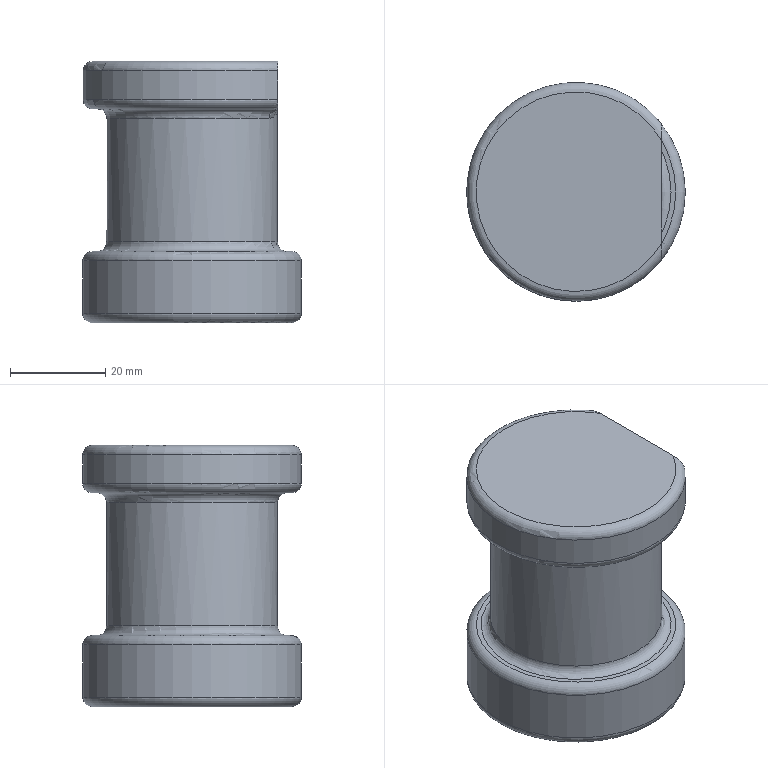Part | NX | features solid 2 | 1 solid | 19 faces | box 46 x 46 x 55 mm | volume 63111 mm3 | torus 6 | plane 5 | cylinder 4 | cone 2 | spline 2 | commonest cylinder face diameters 46 x2 14 x1 36 x1
STEP:
#1=CARTESIAN_POINT('',(458.,215.682,102.));
#2=VERTEX_POINT('',#1);
#3=CARTESIAN_POINT('',(458.,215.682,108.));
#4=VERTEX_POINT('',#3);
#5=CARTESIAN_POINT('',(458.,215.682,110.));
#6=DIRECTION('',(0.,0.,-1.));
#7=VECTOR('',#6,1000.);
#8=LINE('',#5,#7);
#9=EDGE_CURVE('',#2,#4,#8,.F.);
#10=ORIENTED_EDGE('',*,*,#9,.T.);
#11=CARTESIAN_POINT('',(458.,244.318,108.));
#12=VERTEX_POINT('',#11);
#13=CARTESIAN_POINT('',(440.,230.,108.));
#14=DIRECTION('',(0.,0.,1.));
#15=DIRECTION('',(1.,0.,0.));
#16=AXIS2_PLACEMENT_3D('',#13,#14,#15);
#17=CIRCLE('',#16,23.);
#18=EDGE_CURVE('',#12,#4,#17,.T.);
#19=ORIENTED_EDGE('',*,*,#18,.F.);
#20=CARTESIAN_POINT('',(458.,244.318,102.));
#21=VERTEX_POINT('',#20);
#22=CARTESIAN_POINT('',(458.,244.318,110.));
#23=DIRECTION('',(0.,0.,-1.));
#24=VECTOR('',#23,1000.);
#25=LINE('',#22,#24);
#26=EDGE_CURVE('',#12,#21,#25,.T.);
#27=ORIENTED_EDGE('',*,*,#26,.T.);
#28=CARTESIAN_POINT('',(440.,230.,102.));
#29=DIRECTION('',(0.,0.,1.));
#30=DIRECTION('',(1.,0.,0.));
#31=AXIS2_PLACEMENT_3D('',#28,#29,#30);
#32=CIRCLE('',#31,23.);
#33=EDGE_CURVE('',#2,#21,#32,.F.);
#34=ORIENTED_EDGE('',*,*,#33,.F.);
#35=EDGE_LOOP('',(#10,#19,#27,#34));
#36=FACE_BOUND('',#35,.T.);
#37=CARTESIAN_POINT('',(440.,230.,55.));
#38=DIRECTION('',(0.,0.,1.));
#39=DIRECTION('',(-1.,0.,0.));
#40=AXIS2_PLACEMENT_3D('',#37,#38,#39);
#41=CYLINDRICAL_SURFACE('',#40,23.);
#42=ADVANCED_FACE('',(#36),#41,.T.);
#43=CARTESIAN_POINT('',(458.,219.183,110.));
#44=VERTEX_POINT('',#43);
#45=CARTESIAN_POINT('',(458.,240.817,110.));
#46=VERTEX_POINT('',#45);
#47=CARTESIAN_POINT('',(458.,215.682,110.));
#48=DIRECTION('',(0.,1.,0.));
#49=VECTOR('',#48,1000.);
#50=LINE('',#47,#49);
#51=EDGE_CURVE('',#44,#46,#50,.T.);
#52=ORIENTED_EDGE('',*,*,#51,.T.);
#53=CARTESIAN_POINT('',(440.,230.,110.));
#54=DIRECTION('',(0.,0.,1.));
#55=DIRECTION('',(1.,0.,0.));
#56=AXIS2_PLACEMENT_3D('',#53,#54,#55);
#57=CIRCLE('',#56,21.);
#58=EDGE_CURVE('',#44,#46,#57,.F.);
#59=ORIENTED_EDGE('',*,*,#58,.F.);
#60=EDGE_LOOP('',(#52,#59));
#61=FACE_BOUND('',#60,.T.);
#62=CARTESIAN_POINT('',(440.,230.,110.));
#63=DIRECTION('',(0.,0.,-1.));
#64=DIRECTION('',(1.,0.,0.));
#65=AXIS2_PLACEMENT_3D('',#62,#63,#64);
#66=PLANE('',#65);
#67=ADVANCED_FACE('',(#61),#66,.F.);
#68=CARTESIAN_POINT('',(458.,219.183,100.));
#69=VERTEX_POINT('',#68);
#70=CARTESIAN_POINT('',(458.,221.282,100.));
#71=VERTEX_POINT('',#70);
#72=CARTESIAN_POINT('',(458.,230.,100.));
#73=DIRECTION('',(0.,1.,0.));
#74=VECTOR('',#73,1000.);
#75=LINE('',#72,#74);
#76=EDGE_CURVE('',#69,#71,#75,.T.);
#77=ORIENTED_EDGE('',*,*,#76,.F.);
#78=CARTESIAN_POINT('',(458.,240.817,100.));
#79=VERTEX_POINT('',#78);
#80=CARTESIAN_POINT('',(440.,230.,100.));
#81=DIRECTION('',(0.,0.,1.));
#82=DIRECTION('',(1.,0.,0.));
#83=AXIS2_PLACEMENT_3D('',#80,#81,#82);
#84=CIRCLE('',#83,21.);
#85=EDGE_CURVE('',#79,#69,#84,.T.);
#86=ORIENTED_EDGE('',*,*,#85,.F.);
#87=CARTESIAN_POINT('',(458.,238.718,100.));
#88=VERTEX_POINT('',#87);
#89=CARTESIAN_POINT('',(458.,230.,100.));
#90=DIRECTION('',(0.,1.,0.));
#91=VECTOR('',#90,1000.);
#92=LINE('',#89,#91);
#93=EDGE_CURVE('',#88,#79,#92,.T.);
#94=ORIENTED_EDGE('',*,*,#93,.F.);
#95=CARTESIAN_POINT('',(440.,230.,100.));
#96=DIRECTION('',(0.,0.,1.));
#97=DIRECTION('',(1.,0.,0.));
#98=AXIS2_PLACEMENT_3D('',#95,#96,#97);
#99=CIRCLE('',#98,20.);
#100=EDGE_CURVE('',#71,#88,#99,.F.);
#101=ORIENTED_EDGE('',*,*,#100,.F.);
#102=EDGE_LOOP('',(#77,#86,#94,#101));
#103=FACE_BOUND('',#102,.T.);
#104=CARTESIAN_POINT('',(440.,230.,100.));
#105=DIRECTION('',(0.,0.,-1.));
#106=DIRECTION('',(0.,-1.,0.));
#107=AXIS2_PLACEMENT_3D('',#104,#105,#106);
#108=PLANE('',#107);
#109=ADVANCED_FACE('',(#103),#108,.T.);
#110=ORIENTED_EDGE('',*,*,#58,.T.);
#111=CARTESIAN_POINT('',(458.,244.318,108.));
#112=CARTESIAN_POINT('',(458.,244.318,108.369));
#113=CARTESIAN_POINT('',(458.,243.958,109.078));
#114=CARTESIAN_POINT('',(458.,242.663,109.852));
#115=CARTESIAN_POINT('',(458.,241.547,110.));
#116=CARTESIAN_POINT('',(458.,240.817,110.));
#117=B_SPLINE_CURVE_WITH_KNOTS('',3,(#111,#112,#113,#114,#115,#116),.UNSPECIFIED.,.F.,.F.,(4,1,1,4),(0.01075,0.01186,0.01296,0.01517),.UNSPECIFIED.);
#118=EDGE_CURVE('',#12,#46,#117,.T.);
#119=ORIENTED_EDGE('',*,*,#118,.F.);
#120=ORIENTED_EDGE('',*,*,#18,.T.);
#121=CARTESIAN_POINT('',(458.,219.183,110.));
#122=CARTESIAN_POINT('',(458.,218.445,110.));
#123=CARTESIAN_POINT('',(458.,217.331,109.849));
#124=CARTESIAN_POINT('',(458.,216.044,109.077));
#125=CARTESIAN_POINT('',(458.,215.682,108.374));
#126=CARTESIAN_POINT('',(458.,215.682,108.));
#127=B_SPLINE_CURVE_WITH_KNOTS('',3,(#121,#122,#123,#124,#125,#126),.UNSPECIFIED.,.F.,.F.,(4,1,1,4),(0.01631,0.01853,0.01964,0.02075),.UNSPECIFIED.);
#128=EDGE_CURVE('',#44,#4,#127,.T.);
#129=ORIENTED_EDGE('',*,*,#128,.F.);
#130=EDGE_LOOP('',(#110,#119,#120,#129));
#131=FACE_BOUND('',#130,.T.);
#132=CARTESIAN_POINT('',(440.,230.,108.));
#133=DIRECTION('',(0.,0.,-1.));
#134=DIRECTION('',(1.,0.,0.));
#135=AXIS2_PLACEMENT_3D('',#132,#133,#134);
#136=TOROIDAL_SURFACE('',#135,21.,2.);
#137=ADVANCED_FACE('',(#131),#136,.T.);
#138=CARTESIAN_POINT('',(460.,230.,70.));
#139=VERTEX_POINT('',#138);
#140=CARTESIAN_POINT('',(440.,230.,70.));
#141=DIRECTION('',(0.,0.,1.));
#142=DIRECTION('',(1.,0.,0.));
#143=AXIS2_PLACEMENT_3D('',#140,#141,#142);
#144=CIRCLE('',#143,20.);
#145=EDGE_CURVE('',#139,#139,#144,.T.);
#146=ORIENTED_EDGE('',*,*,#145,.F.);
#147=EDGE_LOOP('',(#146));
#148=FACE_BOUND('',#147,.T.);
#149=CARTESIAN_POINT('',(461.,230.,70.));
#150=VERTEX_POINT('',#149);
#151=CARTESIAN_POINT('',(440.,230.,70.));
#152=DIRECTION('',(0.,0.,1.));
#153=DIRECTION('',(1.,0.,0.));
#154=AXIS2_PLACEMENT_3D('',#151,#152,#153);
#155=CIRCLE('',#154,21.);
#156=EDGE_CURVE('',#150,#150,#155,.F.);
#157=ORIENTED_EDGE('',*,*,#156,.F.);
#158=EDGE_LOOP('',(#157));
#159=FACE_BOUND('',#158,.T.);
#160=CARTESIAN_POINT('',(440.,230.,70.));
#161=DIRECTION('',(0.,0.,-1.));
#162=DIRECTION('',(0.,-1.,0.));
#163=AXIS2_PLACEMENT_3D('',#160,#161,#162);
#164=PLANE('',#163);
#165=ADVANCED_FACE('',(#148,#159),#164,.F.);
#166=CARTESIAN_POINT('',(458.,230.,72.));
#167=VERTEX_POINT('',#166);
#168=CARTESIAN_POINT('',(440.,230.,72.));
#169=DIRECTION('',(0.,0.,1.));
#170=DIRECTION('',(1.,0.,0.));
#171=AXIS2_PLACEMENT_3D('',#168,#169,#170);
#172=CIRCLE('',#171,18.);
#173=EDGE_CURVE('',#167,#167,#172,.F.);
#174=ORIENTED_EDGE('',*,*,#173,.F.);
#175=EDGE_LOOP('',(#174));
#176=FACE_BOUND('',#175,.T.);
#177=CARTESIAN_POINT('',(456.2,222.154,98.));
#178=VERTEX_POINT('',#177);
#179=CARTESIAN_POINT('',(458.,230.,100.));
#180=VERTEX_POINT('',#179);
#181=CARTESIAN_POINT('',(456.2,222.154,98.));
#182=CARTESIAN_POINT('',(456.817,223.428,98.));
#183=CARTESIAN_POINT('',(457.712,226.043,98.614));
#184=CARTESIAN_POINT('',(458.,228.665,99.531));
#185=CARTESIAN_POINT('',(458.,230.,100.));
#186=B_SPLINE_CURVE_WITH_KNOTS('',3,(#181,#182,#183,#184,#185),.UNSPECIFIED.,.F.,.F.,(4,1,4),(0.,0.004245,0.00849),.UNSPECIFIED.);
#187=EDGE_CURVE('',#178,#180,#186,.T.);
#188=ORIENTED_EDGE('',*,*,#187,.F.);
#189=CARTESIAN_POINT('',(456.2,237.846,98.));
#190=VERTEX_POINT('',#189);
#191=CARTESIAN_POINT('',(440.,230.,98.));
#192=DIRECTION('',(0.,0.,1.));
#193=DIRECTION('',(1.,0.,0.));
#194=AXIS2_PLACEMENT_3D('',#191,#192,#193);
#195=CIRCLE('',#194,18.);
#196=EDGE_CURVE('',#190,#178,#195,.T.);
#197=ORIENTED_EDGE('',*,*,#196,.F.);
#198=CARTESIAN_POINT('',(456.2,237.846,98.));
#199=CARTESIAN_POINT('',(456.817,236.572,98.));
#200=CARTESIAN_POINT('',(457.712,233.957,98.614));
#201=CARTESIAN_POINT('',(458.,231.335,99.531));
#202=CARTESIAN_POINT('',(458.,230.,100.));
#203=B_SPLINE_CURVE_WITH_KNOTS('',3,(#198,#199,#200,#201,#202),.UNSPECIFIED.,.F.,.F.,(4,1,4),(0.,0.004245,0.00849),.UNSPECIFIED.);
#204=EDGE_CURVE('',#180,#190,#203,.F.);
#205=ORIENTED_EDGE('',*,*,#204,.F.);
#206=EDGE_LOOP('',(#188,#197,#205));
#207=FACE_BOUND('',#206,.T.);
#208=CARTESIAN_POINT('',(440.,230.,85.));
#209=DIRECTION('',(0.,0.,-1.));
#210=DIRECTION('',(0.,-1.,0.));
#211=AXIS2_PLACEMENT_3D('',#208,#209,#210);
#212=CYLINDRICAL_SURFACE('',#211,18.);
#213=ADVANCED_FACE('',(#176,#207),#212,.T.);
#214=CARTESIAN_POINT('',(461.,230.,55.));
#215=VERTEX_POINT('',#214);
#216=CARTESIAN_POINT('',(440.,230.,55.));
#217=DIRECTION('',(0.,0.,1.));
#218=DIRECTION('',(1.,0.,0.));
#219=AXIS2_PLACEMENT_3D('',#216,#217,#218);
#220=CIRCLE('',#219,21.);
#221=EDGE_CURVE('',#215,#215,#220,.T.);
#222=ORIENTED_EDGE('',*,*,#221,.F.);
#223=EDGE_LOOP('',(#222));
#224=FACE_BOUND('',#223,.T.);
#225=CARTESIAN_POINT('',(429.,230.,55.));
#226=VERTEX_POINT('',#225);
#227=CARTESIAN_POINT('',(440.,230.,55.));
#228=DIRECTION('',(0.,0.,-1.));
#229=DIRECTION('',(-1.,0.,0.));
#230=AXIS2_PLACEMENT_3D('',#227,#228,#229);
#231=CIRCLE('',#230,11.);
#232=EDGE_CURVE('',#226,#226,#231,.T.);
#233=ORIENTED_EDGE('',*,*,#232,.F.);
#234=EDGE_LOOP('',(#233));
#235=FACE_BOUND('',#234,.T.);
#236=CARTESIAN_POINT('',(440.,230.,55.));
#237=DIRECTION('',(0.,0.,-1.));
#238=DIRECTION('',(1.,0.,0.));
#239=AXIS2_PLACEMENT_3D('',#236,#237,#238);
#240=PLANE('',#239);
#241=ADVANCED_FACE('',(#224,#235),#240,.T.);
#242=CARTESIAN_POINT('',(463.,230.,57.));
#243=VERTEX_POINT('',#242);
#244=CARTESIAN_POINT('',(440.,230.,57.));
#245=DIRECTION('',(0.,0.,1.));
#246=DIRECTION('',(1.,0.,0.));
#247=AXIS2_PLACEMENT_3D('',#244,#245,#246);
#248=CIRCLE('',#247,23.);
#249=EDGE_CURVE('',#243,#243,#248,.F.);
#250=ORIENTED_EDGE('',*,*,#249,.F.);
#251=EDGE_LOOP('',(#250));
#252=FACE_BOUND('',#251,.T.);
#253=CARTESIAN_POINT('',(463.,230.,68.));
#254=VERTEX_POINT('',#253);
#255=CARTESIAN_POINT('',(440.,230.,68.));
#256=DIRECTION('',(0.,0.,1.));
#257=DIRECTION('',(1.,0.,0.));
#258=AXIS2_PLACEMENT_3D('',#255,#256,#257);
#259=CIRCLE('',#258,23.);
#260=EDGE_CURVE('',#254,#254,#259,.T.);
#261=ORIENTED_EDGE('',*,*,#260,.F.);
#262=EDGE_LOOP('',(#261));
#263=FACE_BOUND('',#262,.T.);
#264=CARTESIAN_POINT('',(440.,230.,55.));
#265=DIRECTION('',(0.,0.,1.));
#266=DIRECTION('',(-1.,0.,0.));
#267=AXIS2_PLACEMENT_3D('',#264,#265,#266);
#268=CYLINDRICAL_SURFACE('',#267,23.);
#269=ADVANCED_FACE('',(#252,#263),#268,.T.);
#270=CARTESIAN_POINT('',(433.,230.,100.));
#271=VERTEX_POINT('',#270);
#272=CARTESIAN_POINT('',(440.,230.,100.));
#273=DIRECTION('',(0.,0.,-1.));
#274=DIRECTION('',(-1.,0.,0.));
#275=AXIS2_PLACEMENT_3D('',#272,#273,#274);
#276=CIRCLE('',#275,7.);
#277=EDGE_CURVE('',#271,#271,#276,.T.);
#278=ORIENTED_EDGE('',*,*,#277,.T.);
#279=EDGE_LOOP('',(#278));
#280=FACE_BOUND('',#279,.T.);
#281=CARTESIAN_POINT('',(440.,230.,101.876));
#282=VERTEX_POINT('',#281);
#283=VERTEX_LOOP('',#282);
#284=FACE_BOUND('',#283,.T.);
#285=CARTESIAN_POINT('',(440.,230.,100.));
#286=DIRECTION('',(0.,0.,-1.));
#287=DIRECTION('',(1.,0.,0.));
#288=AXIS2_PLACEMENT_3D('',#285,#286,#287);
#289=CONICAL_SURFACE('',#288,7.,1.309);
#290=ADVANCED_FACE('',(#280,#284),#289,.F.);
#291=ORIENTED_EDGE('',*,*,#277,.F.);
#292=EDGE_LOOP('',(#291));
#293=FACE_BOUND('',#292,.T.);
#294=CARTESIAN_POINT('',(433.,230.,61.928));
#295=VERTEX_POINT('',#294);
#296=CARTESIAN_POINT('',(440.,230.,61.928));
#297=DIRECTION('',(0.,0.,-1.));
#298=DIRECTION('',(-1.,0.,0.));
#299=AXIS2_PLACEMENT_3D('',#296,#297,#298);
#300=CIRCLE('',#299,7.);
#301=EDGE_CURVE('',#295,#295,#300,.T.);
#302=ORIENTED_EDGE('',*,*,#301,.T.);
#303=EDGE_LOOP('',(#302));
#304=FACE_BOUND('',#303,.T.);
#305=CARTESIAN_POINT('',(440.,230.,100.));
#306=DIRECTION('',(0.,0.,1.));
#307=DIRECTION('',(-1.,0.,0.));
#308=AXIS2_PLACEMENT_3D('',#305,#306,#307);
#309=CYLINDRICAL_SURFACE('',#308,7.);
#310=ADVANCED_FACE('',(#293,#304),#309,.F.);
#311=ORIENTED_EDGE('',*,*,#301,.F.);
#312=EDGE_LOOP('',(#311));
#313=FACE_BOUND('',#312,.T.);
#314=ORIENTED_EDGE('',*,*,#232,.T.);
#315=EDGE_LOOP('',(#314));
#316=FACE_BOUND('',#315,.T.);
#317=CARTESIAN_POINT('',(440.,230.,55.));
#318=DIRECTION('',(0.,0.,-1.));
#319=DIRECTION('',(1.,0.,0.));
#320=AXIS2_PLACEMENT_3D('',#317,#318,#319);
#321=CONICAL_SURFACE('',#320,11.,0.5236);
#322=ADVANCED_FACE('',(#313,#316),#321,.F.);
#323=ORIENTED_EDGE('',*,*,#76,.T.);
#324=CARTESIAN_POINT('',(458.,230.,100.));
#325=DIRECTION('',(0.,1.,0.));
#326=VECTOR('',#325,1000.);
#327=LINE('',#324,#326);
#328=EDGE_CURVE('',#71,#180,#327,.T.);
#329=ORIENTED_EDGE('',*,*,#328,.T.);
#330=CARTESIAN_POINT('',(458.,230.,100.));
#331=DIRECTION('',(0.,1.,0.));
#332=VECTOR('',#331,1000.);
#333=LINE('',#330,#332);
#334=EDGE_CURVE('',#180,#88,#333,.T.);
#335=ORIENTED_EDGE('',*,*,#334,.T.);
#336=ORIENTED_EDGE('',*,*,#93,.T.);
#337=CARTESIAN_POINT('',(458.,244.318,102.));
#338=CARTESIAN_POINT('',(458.,244.318,101.625));
#339=CARTESIAN_POINT('',(458.,243.959,100.927));
#340=CARTESIAN_POINT('',(458.,242.668,100.149));
#341=CARTESIAN_POINT('',(458.,241.556,100.));
#342=CARTESIAN_POINT('',(458.,240.817,100.));
#343=B_SPLINE_CURVE_WITH_KNOTS('',3,(#337,#338,#339,#340,#341,#342),.UNSPECIFIED.,.F.,.F.,(4,1,1,4),(0.,0.001103,0.002207,0.004413),.UNSPECIFIED.);
#344=EDGE_CURVE('',#21,#79,#343,.T.);
#345=ORIENTED_EDGE('',*,*,#344,.F.);
#346=ORIENTED_EDGE('',*,*,#26,.F.);
#347=ORIENTED_EDGE('',*,*,#118,.T.);
#348=ORIENTED_EDGE('',*,*,#51,.F.);
#349=ORIENTED_EDGE('',*,*,#128,.T.);
#350=ORIENTED_EDGE('',*,*,#9,.F.);
#351=CARTESIAN_POINT('',(458.,219.183,100.));
#352=CARTESIAN_POINT('',(458.,218.444,100.));
#353=CARTESIAN_POINT('',(458.,217.342,100.145));
#354=CARTESIAN_POINT('',(458.,216.042,100.925));
#355=CARTESIAN_POINT('',(458.,215.682,101.625));
#356=CARTESIAN_POINT('',(458.,215.682,102.));
#357=B_SPLINE_CURVE_WITH_KNOTS('',3,(#351,#352,#353,#354,#355,#356),.UNSPECIFIED.,.F.,.F.,(4,1,1,4),(0.,0.002188,0.003282,0.004376),.UNSPECIFIED.);
#358=EDGE_CURVE('',#69,#2,#357,.T.);
#359=ORIENTED_EDGE('',*,*,#358,.F.);
#360=EDGE_LOOP('',(#323,#329,#335,#336,#345,#346,#347,#348,#349,#350,#359));
#361=FACE_BOUND('',#360,.T.);
#362=CARTESIAN_POINT('',(458.,215.682,110.));
#363=DIRECTION('',(1.,0.,0.));
#364=DIRECTION('',(0.,0.,1.));
#365=AXIS2_PLACEMENT_3D('',#362,#363,#364);
#366=PLANE('',#365);
#367=ADVANCED_FACE('',(#361),#366,.T.);
#368=ORIENTED_EDGE('',*,*,#249,.T.);
#369=EDGE_LOOP('',(#368));
#370=FACE_BOUND('',#369,.T.);
#371=ORIENTED_EDGE('',*,*,#221,.T.);
#372=EDGE_LOOP('',(#371));
#373=FACE_BOUND('',#372,.T.);
#374=CARTESIAN_POINT('',(440.,230.,57.));
#375=DIRECTION('',(0.,0.,-1.));
#376=DIRECTION('',(1.,0.,0.));
#377=AXIS2_PLACEMENT_3D('',#374,#375,#376);
#378=TOROIDAL_SURFACE('',#377,21.,2.);
#379=ADVANCED_FACE('',(#370,#373),#378,.T.);
#380=ORIENTED_EDGE('',*,*,#328,.F.);
#381=CARTESIAN_POINT('',(458.,221.282,98.));
#382=DIRECTION('',(0.4359,0.9,0.));
#383=DIRECTION('',(-0.9,0.4359,0.));
#384=AXIS2_PLACEMENT_3D('',#381,#382,#383);
#385=CIRCLE('',#384,2.);
#386=EDGE_CURVE('',#71,#178,#385,.F.);
#387=ORIENTED_EDGE('',*,*,#386,.T.);
#388=ORIENTED_EDGE('',*,*,#187,.T.);
#389=EDGE_LOOP('',(#380,#387,#388));
#390=FACE_BOUND('',#389,.T.);
#391=CARTESIAN_POINT('',(458.,221.282,100.));
#392=CARTESIAN_POINT('',(456.2,222.154,100.));
#393=CARTESIAN_POINT('',(456.2,222.154,98.));
#394=CARTESIAN_POINT('',(458.,222.683,100.));
#395=CARTESIAN_POINT('',(456.618,223.017,99.47));
#396=CARTESIAN_POINT('',(456.81,223.414,98.));
#397=CARTESIAN_POINT('',(458.,225.584,100.));
#398=CARTESIAN_POINT('',(457.644,225.617,99.263));
#399=CARTESIAN_POINT('',(457.709,226.026,98.608));
#400=CARTESIAN_POINT('',(458.,228.515,100.));
#401=CARTESIAN_POINT('',(458.,228.59,99.765));
#402=CARTESIAN_POINT('',(458.,228.664,99.531));
#403=CARTESIAN_POINT('',(458.,230.,100.));
#404=CARTESIAN_POINT('',(458.,230.,100.));
#405=CARTESIAN_POINT('',(458.,230.,100.));
#406=(BOUNDED_SURFACE()B_SPLINE_SURFACE(3,2,((#391,#392,#393),(#394,#395,#396),(#397,#398,#399),(#400,#401,#402),(#403,#404,#405)),.UNSPECIFIED.,.F.,.F.,.F.)B_SPLINE_SURFACE_WITH_KNOTS((4,1,4),(3,3),(0.004746,0.009418,0.01409),(0.,1.),.UNSPECIFIED.)GEOMETRIC_REPRESENTATION_ITEM()RATIONAL_B_SPLINE_SURFACE(((1.,0.7071,1.),(1.,0.815,1.),(1.,0.9556,1.),(1.,1.,1.),(1.,1.,1.)))REPRESENTATION_ITEM('')SURFACE());
#407=ADVANCED_FACE('',(#390),#406,.F.);
#408=ORIENTED_EDGE('',*,*,#386,.F.);
#409=ORIENTED_EDGE('',*,*,#100,.T.);
#410=CARTESIAN_POINT('',(458.,238.718,98.));
#411=DIRECTION('',(0.4359,-0.9,0.));
#412=DIRECTION('',(0.9,0.4359,0.));
#413=AXIS2_PLACEMENT_3D('',#410,#411,#412);
#414=CIRCLE('',#413,2.);
#415=EDGE_CURVE('',#88,#190,#414,.T.);
#416=ORIENTED_EDGE('',*,*,#415,.T.);
#417=ORIENTED_EDGE('',*,*,#196,.T.);
#418=EDGE_LOOP('',(#408,#409,#416,#417));
#419=FACE_BOUND('',#418,.T.);
#420=CARTESIAN_POINT('',(440.,230.,98.));
#421=DIRECTION('',(0.,0.,-1.));
#422=DIRECTION('',(1.,0.,0.));
#423=AXIS2_PLACEMENT_3D('',#420,#421,#422);
#424=TOROIDAL_SURFACE('',#423,20.,2.);
#425=ADVANCED_FACE('',(#419),#424,.F.);
#426=ORIENTED_EDGE('',*,*,#204,.T.);
#427=ORIENTED_EDGE('',*,*,#415,.F.);
#428=ORIENTED_EDGE('',*,*,#334,.F.);
#429=EDGE_LOOP('',(#426,#427,#428));
#430=FACE_BOUND('',#429,.T.);
#431=CARTESIAN_POINT('',(456.2,237.846,98.));
#432=CARTESIAN_POINT('',(456.2,237.846,100.));
#433=CARTESIAN_POINT('',(458.,238.718,100.));
#434=CARTESIAN_POINT('',(456.81,236.586,98.));
#435=CARTESIAN_POINT('',(456.618,236.983,99.47));
#436=CARTESIAN_POINT('',(458.,237.317,100.));
#437=CARTESIAN_POINT('',(457.709,233.974,98.608));
#438=CARTESIAN_POINT('',(457.644,234.383,99.263));
#439=CARTESIAN_POINT('',(458.,234.416,100.));
#440=CARTESIAN_POINT('',(458.,231.336,99.531));
#441=CARTESIAN_POINT('',(458.,231.41,99.765));
#442=CARTESIAN_POINT('',(458.,231.485,100.));
#443=CARTESIAN_POINT('',(458.,230.,100.));
#444=CARTESIAN_POINT('',(458.,230.,100.));
#445=CARTESIAN_POINT('',(458.,230.,100.));
#446=(BOUNDED_SURFACE()B_SPLINE_SURFACE(3,2,((#431,#432,#433),(#434,#435,#436),(#437,#438,#439),(#440,#441,#442),(#443,#444,#445)),.UNSPECIFIED.,.F.,.F.,.F.)B_SPLINE_SURFACE_WITH_KNOTS((4,1,4),(3,3),(0.004746,0.009418,0.01409),(0.,1.),.UNSPECIFIED.)GEOMETRIC_REPRESENTATION_ITEM()RATIONAL_B_SPLINE_SURFACE(((1.,0.7071,1.),(1.,0.815,1.),(1.,0.9556,1.),(1.,1.,1.),(1.,1.,1.)))REPRESENTATION_ITEM('')SURFACE());
#447=ADVANCED_FACE('',(#430),#446,.F.);
#448=ORIENTED_EDGE('',*,*,#344,.T.);
#449=ORIENTED_EDGE('',*,*,#85,.T.);
#450=ORIENTED_EDGE('',*,*,#358,.T.);
#451=ORIENTED_EDGE('',*,*,#33,.T.);
#452=EDGE_LOOP('',(#448,#449,#450,#451));
#453=FACE_BOUND('',#452,.T.);
#454=CARTESIAN_POINT('',(440.,230.,102.));
#455=DIRECTION('',(0.,0.,-1.));
#456=DIRECTION('',(1.,0.,0.));
#457=AXIS2_PLACEMENT_3D('',#454,#455,#456);
#458=TOROIDAL_SURFACE('',#457,21.,2.);
#459=ADVANCED_FACE('',(#453),#458,.T.);
#460=ORIENTED_EDGE('',*,*,#173,.T.);
#461=EDGE_LOOP('',(#460));
#462=FACE_BOUND('',#461,.T.);
#463=ORIENTED_EDGE('',*,*,#145,.T.);
#464=EDGE_LOOP('',(#463));
#465=FACE_BOUND('',#464,.T.);
#466=CARTESIAN_POINT('',(440.,230.,72.));
#467=DIRECTION('',(0.,0.,-1.));
#468=DIRECTION('',(1.,0.,0.));
#469=AXIS2_PLACEMENT_3D('',#466,#467,#468);
#470=TOROIDAL_SURFACE('',#469,20.,2.);
#471=ADVANCED_FACE('',(#462,#465),#470,.F.);
#472=ORIENTED_EDGE('',*,*,#156,.T.);
#473=EDGE_LOOP('',(#472));
#474=FACE_BOUND('',#473,.T.);
#475=ORIENTED_EDGE('',*,*,#260,.T.);
#476=EDGE_LOOP('',(#475));
#477=FACE_BOUND('',#476,.T.);
#478=CARTESIAN_POINT('',(440.,230.,68.));
#479=DIRECTION('',(0.,0.,-1.));
#480=DIRECTION('',(1.,0.,0.));
#481=AXIS2_PLACEMENT_3D('',#478,#479,#480);
#482=TOROIDAL_SURFACE('',#481,21.,2.);
#483=ADVANCED_FACE('',(#474,#477),#482,.T.);
#484=CLOSED_SHELL('',(#42,#67,#109,#137,#165,#213,#241,#269,#290,#310,#322,#367,#379,#407,#425,#447,#459,#471,#483));
#485=MANIFOLD_SOLID_BREP('',#484);
#486=(LENGTH_UNIT()NAMED_UNIT(*)SI_UNIT(.MILLI.,.METRE.));
#487=UNCERTAINTY_MEASURE_WITH_UNIT(LENGTH_MEASURE(0.0508),#486,'','');
#488=(NAMED_UNIT(*)PLANE_ANGLE_UNIT()SI_UNIT($,.RADIAN.));
#489=(NAMED_UNIT(*)SI_UNIT($,.STERADIAN.)SOLID_ANGLE_UNIT());
#490=(GEOMETRIC_REPRESENTATION_CONTEXT(3)GLOBAL_UNCERTAINTY_ASSIGNED_CONTEXT((#487))GLOBAL_UNIT_ASSIGNED_CONTEXT((#486,#488,#489))REPRESENTATION_CONTEXT('',''));
#491=ADVANCED_BREP_SHAPE_REPRESENTATION('',(#485),#490);